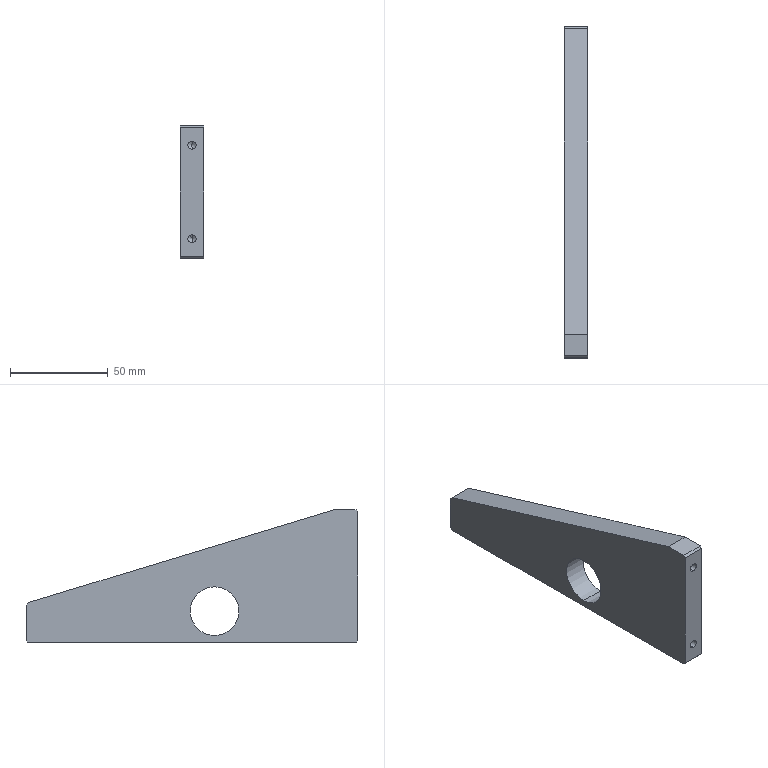Part | SolidWorks | features HoleWzd 2, Chamfer 1, Extrusion 1, ICE 1 | 1 solid | 29 faces | box 12 x 170 x 68 mm | volume 86588 mm3 | plane 11 | cylinder 10 | cone 8 | commonest cylinder face diameters 4.2 x8 25 x2
STEP:
#1=CARTESIAN_POINT('',(-6.,73.4,28.5));
#2=VERTEX_POINT('',#1);
#3=CARTESIAN_POINT('',(-6.,73.4,3.5));
#4=VERTEX_POINT('',#3);
#5=CARTESIAN_POINT('',(-6.,73.4,16.));
#6=DIRECTION('',(1.,0.,0.));
#7=DIRECTION('',(0.,0.,-1.));
#8=AXIS2_PLACEMENT_3D('',#5,#6,#7);
#9=CIRCLE('',#8,12.5);
#10=EDGE_CURVE('',#2,#4,#9,.T.);
#11=ORIENTED_EDGE('',*,*,#10,.F.);
#12=CARTESIAN_POINT('',(6.,73.4,28.5));
#13=VERTEX_POINT('',#12);
#14=CARTESIAN_POINT('',(-6.,73.4,28.5));
#15=DIRECTION('',(1.,0.,0.));
#16=VECTOR('',#15,1000.);
#17=LINE('',#14,#16);
#18=EDGE_CURVE('',#2,#13,#17,.T.);
#19=ORIENTED_EDGE('',*,*,#18,.T.);
#20=CARTESIAN_POINT('',(6.,73.4,3.5));
#21=VERTEX_POINT('',#20);
#22=CARTESIAN_POINT('',(6.,73.4,16.));
#23=DIRECTION('',(1.,0.,0.));
#24=DIRECTION('',(0.,0.,-1.));
#25=AXIS2_PLACEMENT_3D('',#22,#23,#24);
#26=CIRCLE('',#25,12.5);
#27=EDGE_CURVE('',#13,#21,#26,.T.);
#28=ORIENTED_EDGE('',*,*,#27,.T.);
#29=CARTESIAN_POINT('',(-6.,73.4,3.5));
#30=DIRECTION('',(1.,0.,0.));
#31=VECTOR('',#30,1000.);
#32=LINE('',#29,#31);
#33=EDGE_CURVE('',#4,#21,#32,.T.);
#34=ORIENTED_EDGE('',*,*,#33,.F.);
#35=EDGE_LOOP('',(#11,#19,#28,#34));
#36=FACE_OUTER_BOUND('',#35,.T.);
#37=CARTESIAN_POINT('',(-6.,73.4,16.));
#38=DIRECTION('',(1.,0.,0.));
#39=DIRECTION('',(0.,0.,-1.));
#40=AXIS2_PLACEMENT_3D('',#37,#38,#39);
#41=CYLINDRICAL_SURFACE('',#40,12.5);
#42=ADVANCED_FACE('',(#36),#41,.F.);
#43=CARTESIAN_POINT('',(0.,12.4,12.1));
#44=VERTEX_POINT('',#43);
#45=CARTESIAN_POINT('',(0.,12.4,7.9));
#46=VERTEX_POINT('',#45);
#47=CARTESIAN_POINT('',(0.,12.4,10.));
#48=DIRECTION('',(0.,-1.,0.));
#49=DIRECTION('',(0.,0.,-1.));
#50=AXIS2_PLACEMENT_3D('',#47,#48,#49);
#51=CIRCLE('',#50,2.1);
#52=EDGE_CURVE('',#44,#46,#51,.T.);
#53=ORIENTED_EDGE('',*,*,#52,.F.);
#54=CARTESIAN_POINT('',(0.,0.,12.1));
#55=VERTEX_POINT('',#54);
#56=CARTESIAN_POINT('',(0.,0.,12.1));
#57=DIRECTION('',(0.,-1.,0.));
#58=VECTOR('',#57,1000.);
#59=LINE('',#56,#58);
#60=EDGE_CURVE('',#44,#55,#59,.T.);
#61=ORIENTED_EDGE('',*,*,#60,.T.);
#62=CARTESIAN_POINT('',(0.,0.,7.9));
#63=VERTEX_POINT('',#62);
#64=CARTESIAN_POINT('',(0.,0.,10.));
#65=DIRECTION('',(0.,-1.,0.));
#66=DIRECTION('',(0.,0.,-1.));
#67=AXIS2_PLACEMENT_3D('',#64,#65,#66);
#68=CIRCLE('',#67,2.1);
#69=EDGE_CURVE('',#55,#63,#68,.T.);
#70=ORIENTED_EDGE('',*,*,#69,.T.);
#71=CARTESIAN_POINT('',(0.,0.,7.9));
#72=DIRECTION('',(0.,-1.,0.));
#73=VECTOR('',#72,1000.);
#74=LINE('',#71,#73);
#75=EDGE_CURVE('',#46,#63,#74,.T.);
#76=ORIENTED_EDGE('',*,*,#75,.F.);
#77=EDGE_LOOP('',(#53,#61,#70,#76));
#78=FACE_OUTER_BOUND('',#77,.T.);
#79=CARTESIAN_POINT('',(0.,0.,10.));
#80=DIRECTION('',(0.,-1.,0.));
#81=DIRECTION('',(0.,0.,-1.));
#82=AXIS2_PLACEMENT_3D('',#79,#80,#81);
#83=CYLINDRICAL_SURFACE('',#82,2.1);
#84=ADVANCED_FACE('',(#78),#83,.F.);
#85=CARTESIAN_POINT('',(0.,13.662,10.));
#86=VERTEX_POINT('',#85);
#87=CARTESIAN_POINT('',(0.,12.4,7.9));
#88=DIRECTION('',(0.,-0.515,-0.8572));
#89=VECTOR('',#88,1000.);
#90=LINE('',#87,#89);
#91=EDGE_CURVE('',#86,#46,#90,.T.);
#92=ORIENTED_EDGE('',*,*,#91,.F.);
#93=CARTESIAN_POINT('',(0.,12.4,12.1));
#94=DIRECTION('',(0.,-0.515,0.8572));
#95=VECTOR('',#94,1000.);
#96=LINE('',#93,#95);
#97=EDGE_CURVE('',#86,#44,#96,.T.);
#98=ORIENTED_EDGE('',*,*,#97,.T.);
#99=ORIENTED_EDGE('',*,*,#52,.T.);
#100=EDGE_LOOP('',(#92,#98,#99));
#101=FACE_OUTER_BOUND('',#100,.T.);
#102=CARTESIAN_POINT('',(0.,12.4,10.));
#103=DIRECTION('',(0.,-1.,0.));
#104=DIRECTION('',(0.,0.,-1.));
#105=AXIS2_PLACEMENT_3D('',#102,#103,#104);
#106=CONICAL_SURFACE('',#105,2.1,1.03);
#107=ADVANCED_FACE('',(#101),#106,.F.);
#108=CARTESIAN_POINT('',(0.,12.4,60.1));
#109=VERTEX_POINT('',#108);
#110=CARTESIAN_POINT('',(0.,12.4,55.9));
#111=VERTEX_POINT('',#110);
#112=CARTESIAN_POINT('',(0.,12.4,58.));
#113=DIRECTION('',(0.,-1.,0.));
#114=DIRECTION('',(0.,0.,-1.));
#115=AXIS2_PLACEMENT_3D('',#112,#113,#114);
#116=CIRCLE('',#115,2.1);
#117=EDGE_CURVE('',#109,#111,#116,.T.);
#118=ORIENTED_EDGE('',*,*,#117,.F.);
#119=CARTESIAN_POINT('',(0.,0.,60.1));
#120=VERTEX_POINT('',#119);
#121=CARTESIAN_POINT('',(0.,0.,60.1));
#122=DIRECTION('',(0.,-1.,0.));
#123=VECTOR('',#122,1000.);
#124=LINE('',#121,#123);
#125=EDGE_CURVE('',#109,#120,#124,.T.);
#126=ORIENTED_EDGE('',*,*,#125,.T.);
#127=CARTESIAN_POINT('',(0.,0.,55.9));
#128=VERTEX_POINT('',#127);
#129=CARTESIAN_POINT('',(0.,0.,58.));
#130=DIRECTION('',(0.,-1.,0.));
#131=DIRECTION('',(0.,0.,-1.));
#132=AXIS2_PLACEMENT_3D('',#129,#130,#131);
#133=CIRCLE('',#132,2.1);
#134=EDGE_CURVE('',#120,#128,#133,.T.);
#135=ORIENTED_EDGE('',*,*,#134,.T.);
#136=CARTESIAN_POINT('',(0.,0.,55.9));
#137=DIRECTION('',(0.,-1.,0.));
#138=VECTOR('',#137,1000.);
#139=LINE('',#136,#138);
#140=EDGE_CURVE('',#111,#128,#139,.T.);
#141=ORIENTED_EDGE('',*,*,#140,.F.);
#142=EDGE_LOOP('',(#118,#126,#135,#141));
#143=FACE_OUTER_BOUND('',#142,.T.);
#144=CARTESIAN_POINT('',(0.,0.,58.));
#145=DIRECTION('',(0.,-1.,0.));
#146=DIRECTION('',(0.,0.,-1.));
#147=AXIS2_PLACEMENT_3D('',#144,#145,#146);
#148=CYLINDRICAL_SURFACE('',#147,2.1);
#149=ADVANCED_FACE('',(#143),#148,.F.);
#150=CARTESIAN_POINT('',(0.,13.662,58.));
#151=VERTEX_POINT('',#150);
#152=CARTESIAN_POINT('',(0.,12.4,55.9));
#153=DIRECTION('',(0.,-0.515,-0.8572));
#154=VECTOR('',#153,1000.);
#155=LINE('',#152,#154);
#156=EDGE_CURVE('',#151,#111,#155,.T.);
#157=ORIENTED_EDGE('',*,*,#156,.F.);
#158=CARTESIAN_POINT('',(0.,12.4,60.1));
#159=DIRECTION('',(0.,-0.515,0.8572));
#160=VECTOR('',#159,1000.);
#161=LINE('',#158,#160);
#162=EDGE_CURVE('',#151,#109,#161,.T.);
#163=ORIENTED_EDGE('',*,*,#162,.T.);
#164=ORIENTED_EDGE('',*,*,#117,.T.);
#165=EDGE_LOOP('',(#157,#163,#164));
#166=FACE_OUTER_BOUND('',#165,.T.);
#167=CARTESIAN_POINT('',(0.,12.4,58.));
#168=DIRECTION('',(0.,-1.,0.));
#169=DIRECTION('',(0.,0.,-1.));
#170=AXIS2_PLACEMENT_3D('',#167,#168,#169);
#171=CONICAL_SURFACE('',#170,2.1,1.03);
#172=ADVANCED_FACE('',(#166),#171,.F.);
#173=CARTESIAN_POINT('',(0.,152.9,12.4));
#174=VERTEX_POINT('',#173);
#175=CARTESIAN_POINT('',(0.,157.1,12.4));
#176=VERTEX_POINT('',#175);
#177=CARTESIAN_POINT('',(0.,155.,12.4));
#178=DIRECTION('',(0.,0.,-1.));
#179=DIRECTION('',(0.,1.,0.));
#180=AXIS2_PLACEMENT_3D('',#177,#178,#179);
#181=CIRCLE('',#180,2.1);
#182=EDGE_CURVE('',#174,#176,#181,.T.);
#183=ORIENTED_EDGE('',*,*,#182,.F.);
#184=CARTESIAN_POINT('',(0.,152.9,0.));
#185=VERTEX_POINT('',#184);
#186=CARTESIAN_POINT('',(0.,152.9,0.));
#187=DIRECTION('',(0.,0.,-1.));
#188=VECTOR('',#187,1000.);
#189=LINE('',#186,#188);
#190=EDGE_CURVE('',#174,#185,#189,.T.);
#191=ORIENTED_EDGE('',*,*,#190,.T.);
#192=CARTESIAN_POINT('',(0.,157.1,0.));
#193=VERTEX_POINT('',#192);
#194=CARTESIAN_POINT('',(0.,155.,0.));
#195=DIRECTION('',(0.,0.,-1.));
#196=DIRECTION('',(0.,1.,0.));
#197=AXIS2_PLACEMENT_3D('',#194,#195,#196);
#198=CIRCLE('',#197,2.1);
#199=EDGE_CURVE('',#185,#193,#198,.T.);
#200=ORIENTED_EDGE('',*,*,#199,.T.);
#201=CARTESIAN_POINT('',(0.,157.1,0.));
#202=DIRECTION('',(0.,0.,-1.));
#203=VECTOR('',#202,1000.);
#204=LINE('',#201,#203);
#205=EDGE_CURVE('',#176,#193,#204,.T.);
#206=ORIENTED_EDGE('',*,*,#205,.F.);
#207=EDGE_LOOP('',(#183,#191,#200,#206));
#208=FACE_OUTER_BOUND('',#207,.T.);
#209=CARTESIAN_POINT('',(0.,155.,0.));
#210=DIRECTION('',(0.,0.,-1.));
#211=DIRECTION('',(0.,1.,0.));
#212=AXIS2_PLACEMENT_3D('',#209,#210,#211);
#213=CYLINDRICAL_SURFACE('',#212,2.1);
#214=ADVANCED_FACE('',(#208),#213,.F.);
#215=CARTESIAN_POINT('',(0.,155.,13.662));
#216=VERTEX_POINT('',#215);
#217=CARTESIAN_POINT('',(0.,157.1,12.4));
#218=DIRECTION('',(0.,0.8572,-0.515));
#219=VECTOR('',#218,1000.);
#220=LINE('',#217,#219);
#221=EDGE_CURVE('',#216,#176,#220,.T.);
#222=ORIENTED_EDGE('',*,*,#221,.F.);
#223=CARTESIAN_POINT('',(0.,152.9,12.4));
#224=DIRECTION('',(0.,-0.8572,-0.515));
#225=VECTOR('',#224,1000.);
#226=LINE('',#223,#225);
#227=EDGE_CURVE('',#216,#174,#226,.T.);
#228=ORIENTED_EDGE('',*,*,#227,.T.);
#229=ORIENTED_EDGE('',*,*,#182,.T.);
#230=EDGE_LOOP('',(#222,#228,#229));
#231=FACE_OUTER_BOUND('',#230,.T.);
#232=CARTESIAN_POINT('',(0.,155.,12.4));
#233=DIRECTION('',(0.,0.,-1.));
#234=DIRECTION('',(0.,1.,0.));
#235=AXIS2_PLACEMENT_3D('',#232,#233,#234);
#236=CONICAL_SURFACE('',#235,2.1,1.03);
#237=ADVANCED_FACE('',(#231),#236,.F.);
#238=CARTESIAN_POINT('',(0.,17.9,12.4));
#239=VERTEX_POINT('',#238);
#240=CARTESIAN_POINT('',(0.,22.1,12.4));
#241=VERTEX_POINT('',#240);
#242=CARTESIAN_POINT('',(0.,20.,12.4));
#243=DIRECTION('',(0.,0.,-1.));
#244=DIRECTION('',(0.,1.,0.));
#245=AXIS2_PLACEMENT_3D('',#242,#243,#244);
#246=CIRCLE('',#245,2.1);
#247=EDGE_CURVE('',#239,#241,#246,.T.);
#248=ORIENTED_EDGE('',*,*,#247,.F.);
#249=CARTESIAN_POINT('',(0.,17.9,0.));
#250=VERTEX_POINT('',#249);
#251=CARTESIAN_POINT('',(0.,17.9,0.));
#252=DIRECTION('',(0.,0.,-1.));
#253=VECTOR('',#252,1000.);
#254=LINE('',#251,#253);
#255=EDGE_CURVE('',#239,#250,#254,.T.);
#256=ORIENTED_EDGE('',*,*,#255,.T.);
#257=CARTESIAN_POINT('',(0.,22.1,0.));
#258=VERTEX_POINT('',#257);
#259=CARTESIAN_POINT('',(0.,20.,0.));
#260=DIRECTION('',(0.,0.,-1.));
#261=DIRECTION('',(0.,1.,0.));
#262=AXIS2_PLACEMENT_3D('',#259,#260,#261);
#263=CIRCLE('',#262,2.1);
#264=EDGE_CURVE('',#250,#258,#263,.T.);
#265=ORIENTED_EDGE('',*,*,#264,.T.);
#266=CARTESIAN_POINT('',(0.,22.1,0.));
#267=DIRECTION('',(0.,0.,-1.));
#268=VECTOR('',#267,1000.);
#269=LINE('',#266,#268);
#270=EDGE_CURVE('',#241,#258,#269,.T.);
#271=ORIENTED_EDGE('',*,*,#270,.F.);
#272=EDGE_LOOP('',(#248,#256,#265,#271));
#273=FACE_OUTER_BOUND('',#272,.T.);
#274=CARTESIAN_POINT('',(0.,20.,0.));
#275=DIRECTION('',(0.,0.,-1.));
#276=DIRECTION('',(0.,1.,0.));
#277=AXIS2_PLACEMENT_3D('',#274,#275,#276);
#278=CYLINDRICAL_SURFACE('',#277,2.1);
#279=ADVANCED_FACE('',(#273),#278,.F.);
#280=CARTESIAN_POINT('',(0.,20.,13.662));
#281=VERTEX_POINT('',#280);
#282=CARTESIAN_POINT('',(0.,22.1,12.4));
#283=DIRECTION('',(0.,0.8572,-0.515));
#284=VECTOR('',#283,1000.);
#285=LINE('',#282,#284);
#286=EDGE_CURVE('',#281,#241,#285,.T.);
#287=ORIENTED_EDGE('',*,*,#286,.F.);
#288=CARTESIAN_POINT('',(0.,17.9,12.4));
#289=DIRECTION('',(0.,-0.8572,-0.515));
#290=VECTOR('',#289,1000.);
#291=LINE('',#288,#290);
#292=EDGE_CURVE('',#281,#239,#291,.T.);
#293=ORIENTED_EDGE('',*,*,#292,.T.);
#294=ORIENTED_EDGE('',*,*,#247,.T.);
#295=EDGE_LOOP('',(#287,#293,#294));
#296=FACE_OUTER_BOUND('',#295,.T.);
#297=CARTESIAN_POINT('',(0.,20.,12.4));
#298=DIRECTION('',(0.,0.,-1.));
#299=DIRECTION('',(0.,1.,0.));
#300=AXIS2_PLACEMENT_3D('',#297,#298,#299);
#301=CONICAL_SURFACE('',#300,2.1,1.03);
#302=ADVANCED_FACE('',(#296),#301,.F.);
#303=CARTESIAN_POINT('',(0.,155.,0.));
#304=DIRECTION('',(0.,0.,-1.));
#305=DIRECTION('',(0.,1.,0.));
#306=AXIS2_PLACEMENT_3D('',#303,#304,#305);
#307=CIRCLE('',#306,2.1);
#308=EDGE_CURVE('',#193,#185,#307,.T.);
#309=ORIENTED_EDGE('',*,*,#308,.F.);
#310=ORIENTED_EDGE('',*,*,#199,.F.);
#311=EDGE_LOOP('',(#309,#310));
#312=FACE_BOUND('',#311,.T.);
#313=CARTESIAN_POINT('',(0.,20.,0.));
#314=DIRECTION('',(0.,0.,-1.));
#315=DIRECTION('',(0.,1.,0.));
#316=AXIS2_PLACEMENT_3D('',#313,#314,#315);
#317=CIRCLE('',#316,2.1);
#318=EDGE_CURVE('',#258,#250,#317,.T.);
#319=ORIENTED_EDGE('',*,*,#318,.F.);
#320=ORIENTED_EDGE('',*,*,#264,.F.);
#321=EDGE_LOOP('',(#319,#320));
#322=FACE_BOUND('',#321,.T.);
#323=CARTESIAN_POINT('',(-6.,1.,0.));
#324=VERTEX_POINT('',#323);
#325=CARTESIAN_POINT('',(-6.,169.,0.));
#326=VERTEX_POINT('',#325);
#327=CARTESIAN_POINT('',(-6.,170.,0.));
#328=DIRECTION('',(0.,1.,0.));
#329=VECTOR('',#328,1000.);
#330=LINE('',#327,#329);
#331=EDGE_CURVE('',#324,#326,#330,.T.);
#332=ORIENTED_EDGE('',*,*,#331,.T.);
#333=CARTESIAN_POINT('',(6.,169.,0.));
#334=VERTEX_POINT('',#333);
#335=CARTESIAN_POINT('',(6.,169.,0.));
#336=DIRECTION('',(1.,0.,0.));
#337=VECTOR('',#336,1000.);
#338=LINE('',#335,#337);
#339=EDGE_CURVE('',#326,#334,#338,.T.);
#340=ORIENTED_EDGE('',*,*,#339,.T.);
#341=CARTESIAN_POINT('',(6.,1.,0.));
#342=VERTEX_POINT('',#341);
#343=CARTESIAN_POINT('',(6.,170.,0.));
#344=DIRECTION('',(0.,1.,0.));
#345=VECTOR('',#344,1000.);
#346=LINE('',#343,#345);
#347=EDGE_CURVE('',#342,#334,#346,.T.);
#348=ORIENTED_EDGE('',*,*,#347,.F.);
#349=CARTESIAN_POINT('',(6.,1.,0.));
#350=DIRECTION('',(-1.,0.,0.));
#351=VECTOR('',#350,1000.);
#352=LINE('',#349,#351);
#353=EDGE_CURVE('',#342,#324,#352,.T.);
#354=ORIENTED_EDGE('',*,*,#353,.T.);
#355=EDGE_LOOP('',(#332,#340,#348,#354));
#356=FACE_OUTER_BOUND('',#355,.T.);
#357=CARTESIAN_POINT('',(6.,170.,0.));
#358=DIRECTION('',(0.,0.,1.));
#359=DIRECTION('',(0.,-1.,0.));
#360=AXIS2_PLACEMENT_3D('',#357,#358,#359);
#361=PLANE('',#360);
#362=ADVANCED_FACE('',(#312,#322,#356),#361,.F.);
#363=CARTESIAN_POINT('',(-6.,170.,1.));
#364=VERTEX_POINT('',#363);
#365=CARTESIAN_POINT('',(-6.,170.,19.));
#366=VERTEX_POINT('',#365);
#367=CARTESIAN_POINT('',(-6.,170.,20.));
#368=DIRECTION('',(0.,0.,1.));
#369=VECTOR('',#368,1000.);
#370=LINE('',#367,#369);
#371=EDGE_CURVE('',#364,#366,#370,.T.);
#372=ORIENTED_EDGE('',*,*,#371,.T.);
#373=CARTESIAN_POINT('',(6.,170.,19.));
#374=VERTEX_POINT('',#373);
#375=CARTESIAN_POINT('',(6.,170.,19.));
#376=DIRECTION('',(1.,0.,0.));
#377=VECTOR('',#376,1000.);
#378=LINE('',#375,#377);
#379=EDGE_CURVE('',#366,#374,#378,.T.);
#380=ORIENTED_EDGE('',*,*,#379,.T.);
#381=CARTESIAN_POINT('',(6.,170.,1.));
#382=VERTEX_POINT('',#381);
#383=CARTESIAN_POINT('',(6.,170.,20.));
#384=DIRECTION('',(0.,0.,1.));
#385=VECTOR('',#384,1000.);
#386=LINE('',#383,#385);
#387=EDGE_CURVE('',#382,#374,#386,.T.);
#388=ORIENTED_EDGE('',*,*,#387,.F.);
#389=CARTESIAN_POINT('',(6.,170.,1.));
#390=DIRECTION('',(-1.,0.,0.));
#391=VECTOR('',#390,1000.);
#392=LINE('',#389,#391);
#393=EDGE_CURVE('',#382,#364,#392,.T.);
#394=ORIENTED_EDGE('',*,*,#393,.T.);
#395=EDGE_LOOP('',(#372,#380,#388,#394));
#396=FACE_OUTER_BOUND('',#395,.T.);
#397=CARTESIAN_POINT('',(6.,170.,20.));
#398=DIRECTION('',(0.,-1.,0.));
#399=DIRECTION('',(0.,0.,-1.));
#400=AXIS2_PLACEMENT_3D('',#397,#398,#399);
#401=PLANE('',#400);
#402=ADVANCED_FACE('',(#396),#401,.F.);
#403=CARTESIAN_POINT('',(6.,168.564,20.436));
#404=VERTEX_POINT('',#403);
#405=CARTESIAN_POINT('',(6.,12.,68.));
#406=VERTEX_POINT('',#405);
#407=CARTESIAN_POINT('',(6.,12.,68.));
#408=DIRECTION('',(0.,-0.9568,0.2907));
#409=VECTOR('',#408,1000.);
#410=LINE('',#407,#409);
#411=EDGE_CURVE('',#404,#406,#410,.T.);
#412=ORIENTED_EDGE('',*,*,#411,.F.);
#413=CARTESIAN_POINT('',(-6.,168.564,20.436));
#414=VERTEX_POINT('',#413);
#415=CARTESIAN_POINT('',(6.,168.564,20.436));
#416=DIRECTION('',(-1.,0.,0.));
#417=VECTOR('',#416,1000.);
#418=LINE('',#415,#417);
#419=EDGE_CURVE('',#404,#414,#418,.T.);
#420=ORIENTED_EDGE('',*,*,#419,.T.);
#421=CARTESIAN_POINT('',(-6.,12.,68.));
#422=VERTEX_POINT('',#421);
#423=CARTESIAN_POINT('',(-6.,12.,68.));
#424=DIRECTION('',(0.,-0.9568,0.2907));
#425=VECTOR('',#424,1000.);
#426=LINE('',#423,#425);
#427=EDGE_CURVE('',#414,#422,#426,.T.);
#428=ORIENTED_EDGE('',*,*,#427,.T.);
#429=CARTESIAN_POINT('',(6.,12.,68.));
#430=DIRECTION('',(-1.,0.,0.));
#431=VECTOR('',#430,1000.);
#432=LINE('',#429,#431);
#433=EDGE_CURVE('',#406,#422,#432,.T.);
#434=ORIENTED_EDGE('',*,*,#433,.F.);
#435=EDGE_LOOP('',(#412,#420,#428,#434));
#436=FACE_OUTER_BOUND('',#435,.T.);
#437=CARTESIAN_POINT('',(6.,12.,68.));
#438=DIRECTION('',(0.,-0.2907,-0.9568));
#439=DIRECTION('',(0.,0.9568,-0.2907));
#440=AXIS2_PLACEMENT_3D('',#437,#438,#439);
#441=PLANE('',#440);
#442=ADVANCED_FACE('',(#436),#441,.F.);
#443=CARTESIAN_POINT('',(-6.,1.,68.));
#444=VERTEX_POINT('',#443);
#445=CARTESIAN_POINT('',(-6.,0.,68.));
#446=DIRECTION('',(0.,-1.,0.));
#447=VECTOR('',#446,1000.);
#448=LINE('',#445,#447);
#449=EDGE_CURVE('',#422,#444,#448,.T.);
#450=ORIENTED_EDGE('',*,*,#449,.T.);
#451=CARTESIAN_POINT('',(6.,1.,68.));
#452=VERTEX_POINT('',#451);
#453=CARTESIAN_POINT('',(6.,1.,68.));
#454=DIRECTION('',(1.,0.,0.));
#455=VECTOR('',#454,1000.);
#456=LINE('',#453,#455);
#457=EDGE_CURVE('',#444,#452,#456,.T.);
#458=ORIENTED_EDGE('',*,*,#457,.T.);
#459=CARTESIAN_POINT('',(6.,0.,68.));
#460=DIRECTION('',(0.,-1.,0.));
#461=VECTOR('',#460,1000.);
#462=LINE('',#459,#461);
#463=EDGE_CURVE('',#406,#452,#462,.T.);
#464=ORIENTED_EDGE('',*,*,#463,.F.);
#465=ORIENTED_EDGE('',*,*,#433,.T.);
#466=EDGE_LOOP('',(#450,#458,#464,#465));
#467=FACE_OUTER_BOUND('',#466,.T.);
#468=CARTESIAN_POINT('',(6.,0.,68.));
#469=DIRECTION('',(0.,0.,-1.));
#470=DIRECTION('',(-1.,0.,0.));
#471=AXIS2_PLACEMENT_3D('',#468,#469,#470);
#472=PLANE('',#471);
#473=ADVANCED_FACE('',(#467),#472,.F.);
#474=CARTESIAN_POINT('',(0.,0.,10.));
#475=DIRECTION('',(0.,-1.,0.));
#476=DIRECTION('',(0.,0.,-1.));
#477=AXIS2_PLACEMENT_3D('',#474,#475,#476);
#478=CIRCLE('',#477,2.1);
#479=EDGE_CURVE('',#63,#55,#478,.T.);
#480=ORIENTED_EDGE('',*,*,#479,.F.);
#481=ORIENTED_EDGE('',*,*,#69,.F.);
#482=EDGE_LOOP('',(#480,#481));
#483=FACE_BOUND('',#482,.T.);
#484=CARTESIAN_POINT('',(0.,0.,58.));
#485=DIRECTION('',(0.,-1.,0.));
#486=DIRECTION('',(0.,0.,-1.));
#487=AXIS2_PLACEMENT_3D('',#484,#485,#486);
#488=CIRCLE('',#487,2.1);
#489=EDGE_CURVE('',#128,#120,#488,.T.);
#490=ORIENTED_EDGE('',*,*,#489,.F.);
#491=ORIENTED_EDGE('',*,*,#134,.F.);
#492=EDGE_LOOP('',(#490,#491));
#493=FACE_BOUND('',#492,.T.);
#494=CARTESIAN_POINT('',(-6.,0.,67.));
#495=VERTEX_POINT('',#494);
#496=CARTESIAN_POINT('',(-6.,0.,1.));
#497=VERTEX_POINT('',#496);
#498=CARTESIAN_POINT('',(-6.,0.,0.));
#499=DIRECTION('',(0.,0.,-1.));
#500=VECTOR('',#499,1000.);
#501=LINE('',#498,#500);
#502=EDGE_CURVE('',#495,#497,#501,.T.);
#503=ORIENTED_EDGE('',*,*,#502,.T.);
#504=CARTESIAN_POINT('',(6.,0.,1.));
#505=VERTEX_POINT('',#504);
#506=CARTESIAN_POINT('',(6.,0.,1.));
#507=DIRECTION('',(1.,0.,0.));
#508=VECTOR('',#507,1000.);
#509=LINE('',#506,#508);
#510=EDGE_CURVE('',#497,#505,#509,.T.);
#511=ORIENTED_EDGE('',*,*,#510,.T.);
#512=CARTESIAN_POINT('',(6.,0.,67.));
#513=VERTEX_POINT('',#512);
#514=CARTESIAN_POINT('',(6.,0.,0.));
#515=DIRECTION('',(0.,0.,-1.));
#516=VECTOR('',#515,1000.);
#517=LINE('',#514,#516);
#518=EDGE_CURVE('',#513,#505,#517,.T.);
#519=ORIENTED_EDGE('',*,*,#518,.F.);
#520=CARTESIAN_POINT('',(6.,0.,67.));
#521=DIRECTION('',(-1.,0.,0.));
#522=VECTOR('',#521,1000.);
#523=LINE('',#520,#522);
#524=EDGE_CURVE('',#513,#495,#523,.T.);
#525=ORIENTED_EDGE('',*,*,#524,.T.);
#526=EDGE_LOOP('',(#503,#511,#519,#525));
#527=FACE_OUTER_BOUND('',#526,.T.);
#528=CARTESIAN_POINT('',(6.,0.,0.));
#529=DIRECTION('',(0.,1.,0.));
#530=DIRECTION('',(0.,0.,1.));
#531=AXIS2_PLACEMENT_3D('',#528,#529,#530);
#532=PLANE('',#531);
#533=ADVANCED_FACE('',(#483,#493,#527),#532,.F.);
#534=CARTESIAN_POINT('',(6.,73.4,16.));
#535=DIRECTION('',(1.,0.,0.));
#536=DIRECTION('',(0.,0.,-1.));
#537=AXIS2_PLACEMENT_3D('',#534,#535,#536);
#538=CIRCLE('',#537,12.5);
#539=EDGE_CURVE('',#21,#13,#538,.T.);
#540=ORIENTED_EDGE('',*,*,#539,.F.);
#541=ORIENTED_EDGE('',*,*,#27,.F.);
#542=EDGE_LOOP('',(#540,#541));
#543=FACE_BOUND('',#542,.T.);
#544=ORIENTED_EDGE('',*,*,#387,.T.);
#545=CARTESIAN_POINT('',(6.,168.564,20.436));
#546=DIRECTION('',(0.,-0.7071,0.7071));
#547=VECTOR('',#546,1000.);
#548=LINE('',#545,#547);
#549=EDGE_CURVE('',#374,#404,#548,.T.);
#550=ORIENTED_EDGE('',*,*,#549,.T.);
#551=ORIENTED_EDGE('',*,*,#411,.T.);
#552=ORIENTED_EDGE('',*,*,#463,.T.);
#553=CARTESIAN_POINT('',(6.,0.,67.));
#554=DIRECTION('',(0.,-0.7071,-0.7071));
#555=VECTOR('',#554,1000.);
#556=LINE('',#553,#555);
#557=EDGE_CURVE('',#452,#513,#556,.T.);
#558=ORIENTED_EDGE('',*,*,#557,.T.);
#559=ORIENTED_EDGE('',*,*,#518,.T.);
#560=CARTESIAN_POINT('',(6.,1.,0.));
#561=DIRECTION('',(0.,0.7071,-0.7071));
#562=VECTOR('',#561,1000.);
#563=LINE('',#560,#562);
#564=EDGE_CURVE('',#505,#342,#563,.T.);
#565=ORIENTED_EDGE('',*,*,#564,.T.);
#566=ORIENTED_EDGE('',*,*,#347,.T.);
#567=CARTESIAN_POINT('',(6.,170.,1.));
#568=DIRECTION('',(0.,0.7071,0.7071));
#569=VECTOR('',#568,1000.);
#570=LINE('',#567,#569);
#571=EDGE_CURVE('',#334,#382,#570,.T.);
#572=ORIENTED_EDGE('',*,*,#571,.T.);
#573=EDGE_LOOP('',(#544,#550,#551,#552,#558,#559,#565,#566,#572));
#574=FACE_OUTER_BOUND('',#573,.T.);
#575=CARTESIAN_POINT('',(6.,0.,0.));
#576=DIRECTION('',(-1.,0.,0.));
#577=DIRECTION('',(0.,0.,1.));
#578=AXIS2_PLACEMENT_3D('',#575,#576,#577);
#579=PLANE('',#578);
#580=ADVANCED_FACE('',(#543,#574),#579,.F.);
#581=CARTESIAN_POINT('',(-6.,73.4,16.));
#582=DIRECTION('',(1.,0.,0.));
#583=DIRECTION('',(0.,0.,-1.));
#584=AXIS2_PLACEMENT_3D('',#581,#582,#583);
#585=CIRCLE('',#584,12.5);
#586=EDGE_CURVE('',#4,#2,#585,.T.);
#587=ORIENTED_EDGE('',*,*,#586,.T.);
#588=ORIENTED_EDGE('',*,*,#10,.T.);
#589=EDGE_LOOP('',(#587,#588));
#590=FACE_BOUND('',#589,.T.);
#591=ORIENTED_EDGE('',*,*,#427,.F.);
#592=CARTESIAN_POINT('',(-6.,94.5,94.5));
#593=DIRECTION('',(0.,0.7071,-0.7071));
#594=VECTOR('',#593,1000.);
#595=LINE('',#592,#594);
#596=EDGE_CURVE('',#414,#366,#595,.T.);
#597=ORIENTED_EDGE('',*,*,#596,.T.);
#598=ORIENTED_EDGE('',*,*,#371,.F.);
#599=CARTESIAN_POINT('',(-6.,84.5,-84.5));
#600=DIRECTION('',(0.,-0.7071,-0.7071));
#601=VECTOR('',#600,1000.);
#602=LINE('',#599,#601);
#603=EDGE_CURVE('',#364,#326,#602,.T.);
#604=ORIENTED_EDGE('',*,*,#603,.T.);
#605=ORIENTED_EDGE('',*,*,#331,.F.);
#606=CARTESIAN_POINT('',(-6.,0.5,0.5));
#607=DIRECTION('',(0.,-0.7071,0.7071));
#608=VECTOR('',#607,1000.);
#609=LINE('',#606,#608);
#610=EDGE_CURVE('',#324,#497,#609,.T.);
#611=ORIENTED_EDGE('',*,*,#610,.T.);
#612=ORIENTED_EDGE('',*,*,#502,.F.);
#613=CARTESIAN_POINT('',(-6.,-33.5,33.5));
#614=DIRECTION('',(0.,0.7071,0.7071));
#615=VECTOR('',#614,1000.);
#616=LINE('',#613,#615);
#617=EDGE_CURVE('',#495,#444,#616,.T.);
#618=ORIENTED_EDGE('',*,*,#617,.T.);
#619=ORIENTED_EDGE('',*,*,#449,.F.);
#620=EDGE_LOOP('',(#591,#597,#598,#604,#605,#611,#612,#618,#619));
#621=FACE_OUTER_BOUND('',#620,.T.);
#622=CARTESIAN_POINT('',(-6.,0.,0.));
#623=DIRECTION('',(-1.,0.,0.));
#624=DIRECTION('',(0.,0.,1.));
#625=AXIS2_PLACEMENT_3D('',#622,#623,#624);
#626=PLANE('',#625);
#627=ADVANCED_FACE('',(#590,#621),#626,.T.);
#628=ORIENTED_EDGE('',*,*,#292,.F.);
#629=ORIENTED_EDGE('',*,*,#286,.T.);
#630=CARTESIAN_POINT('',(0.,20.,12.4));
#631=DIRECTION('',(0.,0.,-1.));
#632=DIRECTION('',(0.,1.,0.));
#633=AXIS2_PLACEMENT_3D('',#630,#631,#632);
#634=CIRCLE('',#633,2.1);
#635=EDGE_CURVE('',#241,#239,#634,.T.);
#636=ORIENTED_EDGE('',*,*,#635,.T.);
#637=EDGE_LOOP('',(#628,#629,#636));
#638=FACE_OUTER_BOUND('',#637,.T.);
#639=CARTESIAN_POINT('',(0.,20.,12.4));
#640=DIRECTION('',(0.,0.,-1.));
#641=DIRECTION('',(0.,1.,0.));
#642=AXIS2_PLACEMENT_3D('',#639,#640,#641);
#643=CONICAL_SURFACE('',#642,2.1,1.03);
#644=ADVANCED_FACE('',(#638),#643,.F.);
#645=ORIENTED_EDGE('',*,*,#255,.F.);
#646=ORIENTED_EDGE('',*,*,#635,.F.);
#647=ORIENTED_EDGE('',*,*,#270,.T.);
#648=ORIENTED_EDGE('',*,*,#318,.T.);
#649=EDGE_LOOP('',(#645,#646,#647,#648));
#650=FACE_OUTER_BOUND('',#649,.T.);
#651=CARTESIAN_POINT('',(0.,20.,0.));
#652=DIRECTION('',(0.,0.,-1.));
#653=DIRECTION('',(0.,1.,0.));
#654=AXIS2_PLACEMENT_3D('',#651,#652,#653);
#655=CYLINDRICAL_SURFACE('',#654,2.1);
#656=ADVANCED_FACE('',(#650),#655,.F.);
#657=ORIENTED_EDGE('',*,*,#227,.F.);
#658=ORIENTED_EDGE('',*,*,#221,.T.);
#659=CARTESIAN_POINT('',(0.,155.,12.4));
#660=DIRECTION('',(0.,0.,-1.));
#661=DIRECTION('',(0.,1.,0.));
#662=AXIS2_PLACEMENT_3D('',#659,#660,#661);
#663=CIRCLE('',#662,2.1);
#664=EDGE_CURVE('',#176,#174,#663,.T.);
#665=ORIENTED_EDGE('',*,*,#664,.T.);
#666=EDGE_LOOP('',(#657,#658,#665));
#667=FACE_OUTER_BOUND('',#666,.T.);
#668=CARTESIAN_POINT('',(0.,155.,12.4));
#669=DIRECTION('',(0.,0.,-1.));
#670=DIRECTION('',(0.,1.,0.));
#671=AXIS2_PLACEMENT_3D('',#668,#669,#670);
#672=CONICAL_SURFACE('',#671,2.1,1.03);
#673=ADVANCED_FACE('',(#667),#672,.F.);
#674=ORIENTED_EDGE('',*,*,#190,.F.);
#675=ORIENTED_EDGE('',*,*,#664,.F.);
#676=ORIENTED_EDGE('',*,*,#205,.T.);
#677=ORIENTED_EDGE('',*,*,#308,.T.);
#678=EDGE_LOOP('',(#674,#675,#676,#677));
#679=FACE_OUTER_BOUND('',#678,.T.);
#680=CARTESIAN_POINT('',(0.,155.,0.));
#681=DIRECTION('',(0.,0.,-1.));
#682=DIRECTION('',(0.,1.,0.));
#683=AXIS2_PLACEMENT_3D('',#680,#681,#682);
#684=CYLINDRICAL_SURFACE('',#683,2.1);
#685=ADVANCED_FACE('',(#679),#684,.F.);
#686=ORIENTED_EDGE('',*,*,#162,.F.);
#687=ORIENTED_EDGE('',*,*,#156,.T.);
#688=CARTESIAN_POINT('',(0.,12.4,58.));
#689=DIRECTION('',(0.,-1.,0.));
#690=DIRECTION('',(0.,0.,-1.));
#691=AXIS2_PLACEMENT_3D('',#688,#689,#690);
#692=CIRCLE('',#691,2.1);
#693=EDGE_CURVE('',#111,#109,#692,.T.);
#694=ORIENTED_EDGE('',*,*,#693,.T.);
#695=EDGE_LOOP('',(#686,#687,#694));
#696=FACE_OUTER_BOUND('',#695,.T.);
#697=CARTESIAN_POINT('',(0.,12.4,58.));
#698=DIRECTION('',(0.,-1.,0.));
#699=DIRECTION('',(0.,0.,-1.));
#700=AXIS2_PLACEMENT_3D('',#697,#698,#699);
#701=CONICAL_SURFACE('',#700,2.1,1.03);
#702=ADVANCED_FACE('',(#696),#701,.F.);
#703=ORIENTED_EDGE('',*,*,#125,.F.);
#704=ORIENTED_EDGE('',*,*,#693,.F.);
#705=ORIENTED_EDGE('',*,*,#140,.T.);
#706=ORIENTED_EDGE('',*,*,#489,.T.);
#707=EDGE_LOOP('',(#703,#704,#705,#706));
#708=FACE_OUTER_BOUND('',#707,.T.);
#709=CARTESIAN_POINT('',(0.,0.,58.));
#710=DIRECTION('',(0.,-1.,0.));
#711=DIRECTION('',(0.,0.,-1.));
#712=AXIS2_PLACEMENT_3D('',#709,#710,#711);
#713=CYLINDRICAL_SURFACE('',#712,2.1);
#714=ADVANCED_FACE('',(#708),#713,.F.);
#715=ORIENTED_EDGE('',*,*,#97,.F.);
#716=ORIENTED_EDGE('',*,*,#91,.T.);
#717=CARTESIAN_POINT('',(0.,12.4,10.));
#718=DIRECTION('',(0.,-1.,0.));
#719=DIRECTION('',(0.,0.,-1.));
#720=AXIS2_PLACEMENT_3D('',#717,#718,#719);
#721=CIRCLE('',#720,2.1);
#722=EDGE_CURVE('',#46,#44,#721,.T.);
#723=ORIENTED_EDGE('',*,*,#722,.T.);
#724=EDGE_LOOP('',(#715,#716,#723));
#725=FACE_OUTER_BOUND('',#724,.T.);
#726=CARTESIAN_POINT('',(0.,12.4,10.));
#727=DIRECTION('',(0.,-1.,0.));
#728=DIRECTION('',(0.,0.,-1.));
#729=AXIS2_PLACEMENT_3D('',#726,#727,#728);
#730=CONICAL_SURFACE('',#729,2.1,1.03);
#731=ADVANCED_FACE('',(#725),#730,.F.);
#732=ORIENTED_EDGE('',*,*,#60,.F.);
#733=ORIENTED_EDGE('',*,*,#722,.F.);
#734=ORIENTED_EDGE('',*,*,#75,.T.);
#735=ORIENTED_EDGE('',*,*,#479,.T.);
#736=EDGE_LOOP('',(#732,#733,#734,#735));
#737=FACE_OUTER_BOUND('',#736,.T.);
#738=CARTESIAN_POINT('',(0.,0.,10.));
#739=DIRECTION('',(0.,-1.,0.));
#740=DIRECTION('',(0.,0.,-1.));
#741=AXIS2_PLACEMENT_3D('',#738,#739,#740);
#742=CYLINDRICAL_SURFACE('',#741,2.1);
#743=ADVANCED_FACE('',(#737),#742,.F.);
#744=ORIENTED_EDGE('',*,*,#549,.F.);
#745=ORIENTED_EDGE('',*,*,#379,.F.);
#746=ORIENTED_EDGE('',*,*,#596,.F.);
#747=ORIENTED_EDGE('',*,*,#419,.F.);
#748=EDGE_LOOP('',(#744,#745,#746,#747));
#749=FACE_OUTER_BOUND('',#748,.T.);
#750=CARTESIAN_POINT('',(6.,168.564,20.436));
#751=DIRECTION('',(0.,-0.7071,-0.7071));
#752=DIRECTION('',(-1.,0.,0.));
#753=AXIS2_PLACEMENT_3D('',#750,#751,#752);
#754=PLANE('',#753);
#755=ADVANCED_FACE('',(#749),#754,.F.);
#756=ORIENTED_EDGE('',*,*,#571,.F.);
#757=ORIENTED_EDGE('',*,*,#339,.F.);
#758=ORIENTED_EDGE('',*,*,#603,.F.);
#759=ORIENTED_EDGE('',*,*,#393,.F.);
#760=EDGE_LOOP('',(#756,#757,#758,#759));
#761=FACE_OUTER_BOUND('',#760,.T.);
#762=CARTESIAN_POINT('',(6.,170.,1.));
#763=DIRECTION('',(0.,-0.7071,0.7071));
#764=DIRECTION('',(-1.,0.,0.));
#765=AXIS2_PLACEMENT_3D('',#762,#763,#764);
#766=PLANE('',#765);
#767=ADVANCED_FACE('',(#761),#766,.F.);
#768=ORIENTED_EDGE('',*,*,#564,.F.);
#769=ORIENTED_EDGE('',*,*,#510,.F.);
#770=ORIENTED_EDGE('',*,*,#610,.F.);
#771=ORIENTED_EDGE('',*,*,#353,.F.);
#772=EDGE_LOOP('',(#768,#769,#770,#771));
#773=FACE_OUTER_BOUND('',#772,.T.);
#774=CARTESIAN_POINT('',(6.,1.,0.));
#775=DIRECTION('',(0.,0.7071,0.7071));
#776=DIRECTION('',(-1.,0.,0.));
#777=AXIS2_PLACEMENT_3D('',#774,#775,#776);
#778=PLANE('',#777);
#779=ADVANCED_FACE('',(#773),#778,.F.);
#780=ORIENTED_EDGE('',*,*,#557,.F.);
#781=ORIENTED_EDGE('',*,*,#457,.F.);
#782=ORIENTED_EDGE('',*,*,#617,.F.);
#783=ORIENTED_EDGE('',*,*,#524,.F.);
#784=EDGE_LOOP('',(#780,#781,#782,#783));
#785=FACE_OUTER_BOUND('',#784,.T.);
#786=CARTESIAN_POINT('',(6.,0.,67.));
#787=DIRECTION('',(0.,0.7071,-0.7071));
#788=DIRECTION('',(-1.,0.,0.));
#789=AXIS2_PLACEMENT_3D('',#786,#787,#788);
#790=PLANE('',#789);
#791=ADVANCED_FACE('',(#785),#790,.F.);
#792=ORIENTED_EDGE('',*,*,#18,.F.);
#793=ORIENTED_EDGE('',*,*,#586,.F.);
#794=ORIENTED_EDGE('',*,*,#33,.T.);
#795=ORIENTED_EDGE('',*,*,#539,.T.);
#796=EDGE_LOOP('',(#792,#793,#794,#795));
#797=FACE_OUTER_BOUND('',#796,.T.);
#798=CARTESIAN_POINT('',(-6.,73.4,16.));
#799=DIRECTION('',(1.,0.,0.));
#800=DIRECTION('',(0.,0.,-1.));
#801=AXIS2_PLACEMENT_3D('',#798,#799,#800);
#802=CYLINDRICAL_SURFACE('',#801,12.5);
#803=ADVANCED_FACE('',(#797),#802,.F.);
#804=CLOSED_SHELL('',(#42,#84,#107,#149,#172,#214,#237,#279,#302,#362,#402,#442,#473,#533,#580,#627,#644,#656,#673,#685,#702,#714,#731,#743,#755,#767,#779,#791,#803));
#805=MANIFOLD_SOLID_BREP('',#804);
#806=CARTESIAN_POINT('',(0.,0.,0.));
#807=DIRECTION('',(0.,0.,1.));
#808=DIRECTION('',(1.,0.,0.));
#809=AXIS2_PLACEMENT_3D('',#806,#807,#808);
#810=(LENGTH_UNIT()NAMED_UNIT(*)SI_UNIT(.MILLI.,.METRE.));
#811=UNCERTAINTY_MEASURE_WITH_UNIT(LENGTH_MEASURE(0.00001),#810,'','');
#812=(NAMED_UNIT(*)PLANE_ANGLE_UNIT()SI_UNIT($,.RADIAN.));
#813=(NAMED_UNIT(*)SI_UNIT($,.STERADIAN.)SOLID_ANGLE_UNIT());
#814=(GEOMETRIC_REPRESENTATION_CONTEXT(3)GLOBAL_UNCERTAINTY_ASSIGNED_CONTEXT((#811))GLOBAL_UNIT_ASSIGNED_CONTEXT((#810,#812,#813))REPRESENTATION_CONTEXT('',''));
#815=ADVANCED_BREP_SHAPE_REPRESENTATION('',(#805,#809),#814);